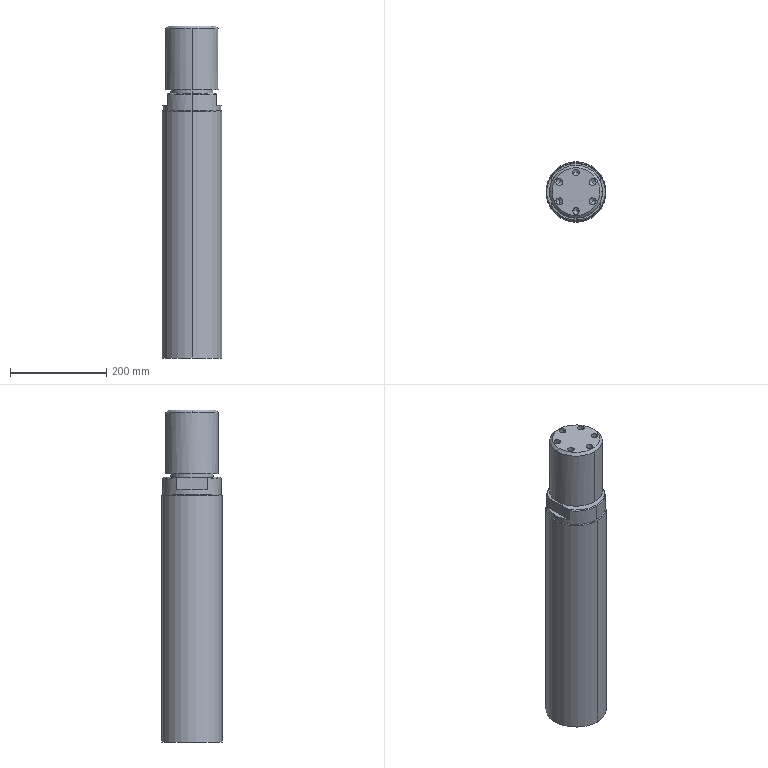Part | SolidWorks | features BaseBody 1, CirPattern 1, HoleWzd 1 | 1 solid | 46 faces | box 125 x 125 x 690 mm | volume 7968385 mm3 | cylinder 20 | cone 18 | plane 8 | commonest cylinder face diameters 14 x12 88 x2 110 x2 121.5 x2 125 x2
STEP:
#1=CARTESIAN_POINT('',(-38.141,13.938,152.));
#2=VERTEX_POINT('',#1);
#3=CARTESIAN_POINT('',(-31.141,26.062,152.));
#4=VERTEX_POINT('',#3);
#5=CARTESIAN_POINT('',(-34.641,20.,152.));
#6=DIRECTION('',(0.,0.,1.));
#7=DIRECTION('',(0.5,0.866,0.));
#8=AXIS2_PLACEMENT_3D('',#5,#6,#7);
#9=CIRCLE('',#8,7.);
#10=EDGE_CURVE('',#2,#4,#9,.T.);
#11=ORIENTED_EDGE('',*,*,#10,.F.);
#12=CARTESIAN_POINT('',(-38.141,13.938,190.));
#13=VERTEX_POINT('',#12);
#14=CARTESIAN_POINT('',(-38.141,13.938,190.));
#15=DIRECTION('',(0.,0.,1.));
#16=VECTOR('',#15,1000.);
#17=LINE('',#14,#16);
#18=EDGE_CURVE('',#2,#13,#17,.T.);
#19=ORIENTED_EDGE('',*,*,#18,.T.);
#20=CARTESIAN_POINT('',(-31.141,26.062,190.));
#21=VERTEX_POINT('',#20);
#22=CARTESIAN_POINT('',(-34.641,20.,190.));
#23=DIRECTION('',(0.,0.,1.));
#24=DIRECTION('',(0.5,0.866,0.));
#25=AXIS2_PLACEMENT_3D('',#22,#23,#24);
#26=CIRCLE('',#25,7.);
#27=EDGE_CURVE('',#13,#21,#26,.T.);
#28=ORIENTED_EDGE('',*,*,#27,.T.);
#29=CARTESIAN_POINT('',(-31.141,26.062,190.));
#30=DIRECTION('',(0.,0.,1.));
#31=VECTOR('',#30,1000.);
#32=LINE('',#29,#31);
#33=EDGE_CURVE('',#4,#21,#32,.T.);
#34=ORIENTED_EDGE('',*,*,#33,.F.);
#35=EDGE_LOOP('',(#11,#19,#28,#34));
#36=FACE_OUTER_BOUND('',#35,.T.);
#37=CARTESIAN_POINT('',(-34.641,20.,190.));
#38=DIRECTION('',(0.,0.,1.));
#39=DIRECTION('',(0.5,0.866,0.));
#40=AXIS2_PLACEMENT_3D('',#37,#38,#39);
#41=CYLINDRICAL_SURFACE('',#40,7.);
#42=ADVANCED_FACE('',(#36),#41,.F.);
#43=CARTESIAN_POINT('',(-34.641,20.,147.794));
#44=VERTEX_POINT('',#43);
#45=CARTESIAN_POINT('',(-31.141,26.062,152.));
#46=DIRECTION('',(0.4286,0.7423,0.515));
#47=VECTOR('',#46,1000.);
#48=LINE('',#45,#47);
#49=EDGE_CURVE('',#44,#4,#48,.T.);
#50=ORIENTED_EDGE('',*,*,#49,.F.);
#51=CARTESIAN_POINT('',(-38.141,13.938,152.));
#52=DIRECTION('',(-0.4286,-0.7423,0.515));
#53=VECTOR('',#52,1000.);
#54=LINE('',#51,#53);
#55=EDGE_CURVE('',#44,#2,#54,.T.);
#56=ORIENTED_EDGE('',*,*,#55,.T.);
#57=ORIENTED_EDGE('',*,*,#10,.T.);
#58=EDGE_LOOP('',(#50,#56,#57));
#59=FACE_OUTER_BOUND('',#58,.T.);
#60=CARTESIAN_POINT('',(-34.641,20.,152.));
#61=DIRECTION('',(0.,0.,1.));
#62=DIRECTION('',(0.5,0.866,0.));
#63=AXIS2_PLACEMENT_3D('',#60,#61,#62);
#64=CONICAL_SURFACE('',#63,7.,1.03);
#65=ADVANCED_FACE('',(#59),#64,.F.);
#66=CARTESIAN_POINT('',(-31.141,-26.062,152.));
#67=VERTEX_POINT('',#66);
#68=CARTESIAN_POINT('',(-38.141,-13.938,152.));
#69=VERTEX_POINT('',#68);
#70=CARTESIAN_POINT('',(-34.641,-20.,152.));
#71=DIRECTION('',(0.,0.,1.));
#72=DIRECTION('',(-0.5,0.866,0.));
#73=AXIS2_PLACEMENT_3D('',#70,#71,#72);
#74=CIRCLE('',#73,7.);
#75=EDGE_CURVE('',#67,#69,#74,.T.);
#76=ORIENTED_EDGE('',*,*,#75,.F.);
#77=CARTESIAN_POINT('',(-31.141,-26.062,190.));
#78=VERTEX_POINT('',#77);
#79=CARTESIAN_POINT('',(-31.141,-26.062,190.));
#80=DIRECTION('',(0.,0.,1.));
#81=VECTOR('',#80,1000.);
#82=LINE('',#79,#81);
#83=EDGE_CURVE('',#67,#78,#82,.T.);
#84=ORIENTED_EDGE('',*,*,#83,.T.);
#85=CARTESIAN_POINT('',(-38.141,-13.938,190.));
#86=VERTEX_POINT('',#85);
#87=CARTESIAN_POINT('',(-34.641,-20.,190.));
#88=DIRECTION('',(0.,0.,1.));
#89=DIRECTION('',(-0.5,0.866,0.));
#90=AXIS2_PLACEMENT_3D('',#87,#88,#89);
#91=CIRCLE('',#90,7.);
#92=EDGE_CURVE('',#78,#86,#91,.T.);
#93=ORIENTED_EDGE('',*,*,#92,.T.);
#94=CARTESIAN_POINT('',(-38.141,-13.938,190.));
#95=DIRECTION('',(0.,0.,1.));
#96=VECTOR('',#95,1000.);
#97=LINE('',#94,#96);
#98=EDGE_CURVE('',#69,#86,#97,.T.);
#99=ORIENTED_EDGE('',*,*,#98,.F.);
#100=EDGE_LOOP('',(#76,#84,#93,#99));
#101=FACE_OUTER_BOUND('',#100,.T.);
#102=CARTESIAN_POINT('',(-34.641,-20.,190.));
#103=DIRECTION('',(0.,0.,1.));
#104=DIRECTION('',(-0.5,0.866,0.));
#105=AXIS2_PLACEMENT_3D('',#102,#103,#104);
#106=CYLINDRICAL_SURFACE('',#105,7.);
#107=ADVANCED_FACE('',(#101),#106,.F.);
#108=CARTESIAN_POINT('',(-34.641,-20.,147.794));
#109=VERTEX_POINT('',#108);
#110=CARTESIAN_POINT('',(-38.141,-13.938,152.));
#111=DIRECTION('',(-0.4286,0.7423,0.515));
#112=VECTOR('',#111,1000.);
#113=LINE('',#110,#112);
#114=EDGE_CURVE('',#109,#69,#113,.T.);
#115=ORIENTED_EDGE('',*,*,#114,.F.);
#116=CARTESIAN_POINT('',(-31.141,-26.062,152.));
#117=DIRECTION('',(0.4286,-0.7423,0.515));
#118=VECTOR('',#117,1000.);
#119=LINE('',#116,#118);
#120=EDGE_CURVE('',#109,#67,#119,.T.);
#121=ORIENTED_EDGE('',*,*,#120,.T.);
#122=ORIENTED_EDGE('',*,*,#75,.T.);
#123=EDGE_LOOP('',(#115,#121,#122));
#124=FACE_OUTER_BOUND('',#123,.T.);
#125=CARTESIAN_POINT('',(-34.641,-20.,152.));
#126=DIRECTION('',(0.,0.,1.));
#127=DIRECTION('',(-0.5,0.866,0.));
#128=AXIS2_PLACEMENT_3D('',#125,#126,#127);
#129=CONICAL_SURFACE('',#128,7.,1.03);
#130=ADVANCED_FACE('',(#124),#129,.F.);
#131=CARTESIAN_POINT('',(7.,-40.,152.));
#132=VERTEX_POINT('',#131);
#133=CARTESIAN_POINT('',(-7.,-40.,152.));
#134=VERTEX_POINT('',#133);
#135=CARTESIAN_POINT('',(0.,-40.,152.));
#136=DIRECTION('',(0.,0.,1.));
#137=DIRECTION('',(-1.,0.,0.));
#138=AXIS2_PLACEMENT_3D('',#135,#136,#137);
#139=CIRCLE('',#138,7.);
#140=EDGE_CURVE('',#132,#134,#139,.T.);
#141=ORIENTED_EDGE('',*,*,#140,.F.);
#142=CARTESIAN_POINT('',(7.,-40.,190.));
#143=VERTEX_POINT('',#142);
#144=CARTESIAN_POINT('',(7.,-40.,190.));
#145=DIRECTION('',(0.,0.,1.));
#146=VECTOR('',#145,1000.);
#147=LINE('',#144,#146);
#148=EDGE_CURVE('',#132,#143,#147,.T.);
#149=ORIENTED_EDGE('',*,*,#148,.T.);
#150=CARTESIAN_POINT('',(-7.,-40.,190.));
#151=VERTEX_POINT('',#150);
#152=CARTESIAN_POINT('',(0.,-40.,190.));
#153=DIRECTION('',(0.,0.,1.));
#154=DIRECTION('',(-1.,0.,0.));
#155=AXIS2_PLACEMENT_3D('',#152,#153,#154);
#156=CIRCLE('',#155,7.);
#157=EDGE_CURVE('',#143,#151,#156,.T.);
#158=ORIENTED_EDGE('',*,*,#157,.T.);
#159=CARTESIAN_POINT('',(-7.,-40.,190.));
#160=DIRECTION('',(0.,0.,1.));
#161=VECTOR('',#160,1000.);
#162=LINE('',#159,#161);
#163=EDGE_CURVE('',#134,#151,#162,.T.);
#164=ORIENTED_EDGE('',*,*,#163,.F.);
#165=EDGE_LOOP('',(#141,#149,#158,#164));
#166=FACE_OUTER_BOUND('',#165,.T.);
#167=CARTESIAN_POINT('',(0.,-40.,190.));
#168=DIRECTION('',(0.,0.,1.));
#169=DIRECTION('',(-1.,0.,0.));
#170=AXIS2_PLACEMENT_3D('',#167,#168,#169);
#171=CYLINDRICAL_SURFACE('',#170,7.);
#172=ADVANCED_FACE('',(#166),#171,.F.);
#173=CARTESIAN_POINT('',(0.,-40.,147.794));
#174=VERTEX_POINT('',#173);
#175=CARTESIAN_POINT('',(-7.,-40.,152.));
#176=DIRECTION('',(-0.8572,0.,0.515));
#177=VECTOR('',#176,1000.);
#178=LINE('',#175,#177);
#179=EDGE_CURVE('',#174,#134,#178,.T.);
#180=ORIENTED_EDGE('',*,*,#179,.F.);
#181=CARTESIAN_POINT('',(7.,-40.,152.));
#182=DIRECTION('',(0.8572,0.,0.515));
#183=VECTOR('',#182,1000.);
#184=LINE('',#181,#183);
#185=EDGE_CURVE('',#174,#132,#184,.T.);
#186=ORIENTED_EDGE('',*,*,#185,.T.);
#187=ORIENTED_EDGE('',*,*,#140,.T.);
#188=EDGE_LOOP('',(#180,#186,#187));
#189=FACE_OUTER_BOUND('',#188,.T.);
#190=CARTESIAN_POINT('',(0.,-40.,152.));
#191=DIRECTION('',(0.,0.,1.));
#192=DIRECTION('',(-1.,0.,0.));
#193=AXIS2_PLACEMENT_3D('',#190,#191,#192);
#194=CONICAL_SURFACE('',#193,7.,1.03);
#195=ADVANCED_FACE('',(#189),#194,.F.);
#196=CARTESIAN_POINT('',(38.141,-13.938,152.));
#197=VERTEX_POINT('',#196);
#198=CARTESIAN_POINT('',(31.141,-26.062,152.));
#199=VERTEX_POINT('',#198);
#200=CARTESIAN_POINT('',(34.641,-20.,152.));
#201=DIRECTION('',(0.,0.,1.));
#202=DIRECTION('',(-0.5,-0.866,0.));
#203=AXIS2_PLACEMENT_3D('',#200,#201,#202);
#204=CIRCLE('',#203,7.);
#205=EDGE_CURVE('',#197,#199,#204,.T.);
#206=ORIENTED_EDGE('',*,*,#205,.F.);
#207=CARTESIAN_POINT('',(38.141,-13.938,190.));
#208=VERTEX_POINT('',#207);
#209=CARTESIAN_POINT('',(38.141,-13.938,190.));
#210=DIRECTION('',(0.,0.,1.));
#211=VECTOR('',#210,1000.);
#212=LINE('',#209,#211);
#213=EDGE_CURVE('',#197,#208,#212,.T.);
#214=ORIENTED_EDGE('',*,*,#213,.T.);
#215=CARTESIAN_POINT('',(31.141,-26.062,190.));
#216=VERTEX_POINT('',#215);
#217=CARTESIAN_POINT('',(34.641,-20.,190.));
#218=DIRECTION('',(0.,0.,1.));
#219=DIRECTION('',(-0.5,-0.866,0.));
#220=AXIS2_PLACEMENT_3D('',#217,#218,#219);
#221=CIRCLE('',#220,7.);
#222=EDGE_CURVE('',#208,#216,#221,.T.);
#223=ORIENTED_EDGE('',*,*,#222,.T.);
#224=CARTESIAN_POINT('',(31.141,-26.062,190.));
#225=DIRECTION('',(0.,0.,1.));
#226=VECTOR('',#225,1000.);
#227=LINE('',#224,#226);
#228=EDGE_CURVE('',#199,#216,#227,.T.);
#229=ORIENTED_EDGE('',*,*,#228,.F.);
#230=EDGE_LOOP('',(#206,#214,#223,#229));
#231=FACE_OUTER_BOUND('',#230,.T.);
#232=CARTESIAN_POINT('',(34.641,-20.,190.));
#233=DIRECTION('',(0.,0.,1.));
#234=DIRECTION('',(-0.5,-0.866,0.));
#235=AXIS2_PLACEMENT_3D('',#232,#233,#234);
#236=CYLINDRICAL_SURFACE('',#235,7.);
#237=ADVANCED_FACE('',(#231),#236,.F.);
#238=CARTESIAN_POINT('',(34.641,-20.,147.794));
#239=VERTEX_POINT('',#238);
#240=CARTESIAN_POINT('',(31.141,-26.062,152.));
#241=DIRECTION('',(-0.4286,-0.7423,0.515));
#242=VECTOR('',#241,1000.);
#243=LINE('',#240,#242);
#244=EDGE_CURVE('',#239,#199,#243,.T.);
#245=ORIENTED_EDGE('',*,*,#244,.F.);
#246=CARTESIAN_POINT('',(38.141,-13.938,152.));
#247=DIRECTION('',(0.4286,0.7423,0.515));
#248=VECTOR('',#247,1000.);
#249=LINE('',#246,#248);
#250=EDGE_CURVE('',#239,#197,#249,.T.);
#251=ORIENTED_EDGE('',*,*,#250,.T.);
#252=ORIENTED_EDGE('',*,*,#205,.T.);
#253=EDGE_LOOP('',(#245,#251,#252));
#254=FACE_OUTER_BOUND('',#253,.T.);
#255=CARTESIAN_POINT('',(34.641,-20.,152.));
#256=DIRECTION('',(0.,0.,1.));
#257=DIRECTION('',(-0.5,-0.866,0.));
#258=AXIS2_PLACEMENT_3D('',#255,#256,#257);
#259=CONICAL_SURFACE('',#258,7.,1.03);
#260=ADVANCED_FACE('',(#254),#259,.F.);
#261=CARTESIAN_POINT('',(31.141,26.062,152.));
#262=VERTEX_POINT('',#261);
#263=CARTESIAN_POINT('',(38.141,13.938,152.));
#264=VERTEX_POINT('',#263);
#265=CARTESIAN_POINT('',(34.641,20.,152.));
#266=DIRECTION('',(0.,0.,1.));
#267=DIRECTION('',(0.5,-0.866,0.));
#268=AXIS2_PLACEMENT_3D('',#265,#266,#267);
#269=CIRCLE('',#268,7.);
#270=EDGE_CURVE('',#262,#264,#269,.T.);
#271=ORIENTED_EDGE('',*,*,#270,.F.);
#272=CARTESIAN_POINT('',(31.141,26.062,190.));
#273=VERTEX_POINT('',#272);
#274=CARTESIAN_POINT('',(31.141,26.062,190.));
#275=DIRECTION('',(0.,0.,1.));
#276=VECTOR('',#275,1000.);
#277=LINE('',#274,#276);
#278=EDGE_CURVE('',#262,#273,#277,.T.);
#279=ORIENTED_EDGE('',*,*,#278,.T.);
#280=CARTESIAN_POINT('',(38.141,13.938,190.));
#281=VERTEX_POINT('',#280);
#282=CARTESIAN_POINT('',(34.641,20.,190.));
#283=DIRECTION('',(0.,0.,1.));
#284=DIRECTION('',(0.5,-0.866,0.));
#285=AXIS2_PLACEMENT_3D('',#282,#283,#284);
#286=CIRCLE('',#285,7.);
#287=EDGE_CURVE('',#273,#281,#286,.T.);
#288=ORIENTED_EDGE('',*,*,#287,.T.);
#289=CARTESIAN_POINT('',(38.141,13.938,190.));
#290=DIRECTION('',(0.,0.,1.));
#291=VECTOR('',#290,1000.);
#292=LINE('',#289,#291);
#293=EDGE_CURVE('',#264,#281,#292,.T.);
#294=ORIENTED_EDGE('',*,*,#293,.F.);
#295=EDGE_LOOP('',(#271,#279,#288,#294));
#296=FACE_OUTER_BOUND('',#295,.T.);
#297=CARTESIAN_POINT('',(34.641,20.,190.));
#298=DIRECTION('',(0.,0.,1.));
#299=DIRECTION('',(0.5,-0.866,0.));
#300=AXIS2_PLACEMENT_3D('',#297,#298,#299);
#301=CYLINDRICAL_SURFACE('',#300,7.);
#302=ADVANCED_FACE('',(#296),#301,.F.);
#303=CARTESIAN_POINT('',(34.641,20.,147.794));
#304=VERTEX_POINT('',#303);
#305=CARTESIAN_POINT('',(38.141,13.938,152.));
#306=DIRECTION('',(0.4286,-0.7423,0.515));
#307=VECTOR('',#306,1000.);
#308=LINE('',#305,#307);
#309=EDGE_CURVE('',#304,#264,#308,.T.);
#310=ORIENTED_EDGE('',*,*,#309,.F.);
#311=CARTESIAN_POINT('',(31.141,26.062,152.));
#312=DIRECTION('',(-0.4286,0.7423,0.515));
#313=VECTOR('',#312,1000.);
#314=LINE('',#311,#313);
#315=EDGE_CURVE('',#304,#262,#314,.T.);
#316=ORIENTED_EDGE('',*,*,#315,.T.);
#317=ORIENTED_EDGE('',*,*,#270,.T.);
#318=EDGE_LOOP('',(#310,#316,#317));
#319=FACE_OUTER_BOUND('',#318,.T.);
#320=CARTESIAN_POINT('',(34.641,20.,152.));
#321=DIRECTION('',(0.,0.,1.));
#322=DIRECTION('',(0.5,-0.866,0.));
#323=AXIS2_PLACEMENT_3D('',#320,#321,#322);
#324=CONICAL_SURFACE('',#323,7.,1.03);
#325=ADVANCED_FACE('',(#319),#324,.F.);
#326=CARTESIAN_POINT('',(-7.,40.,152.));
#327=VERTEX_POINT('',#326);
#328=CARTESIAN_POINT('',(7.,40.,152.));
#329=VERTEX_POINT('',#328);
#330=CARTESIAN_POINT('',(0.,40.,152.));
#331=DIRECTION('',(0.,0.,1.));
#332=DIRECTION('',(1.,0.,0.));
#333=AXIS2_PLACEMENT_3D('',#330,#331,#332);
#334=CIRCLE('',#333,7.);
#335=EDGE_CURVE('',#327,#329,#334,.T.);
#336=ORIENTED_EDGE('',*,*,#335,.F.);
#337=CARTESIAN_POINT('',(-7.,40.,190.));
#338=VERTEX_POINT('',#337);
#339=CARTESIAN_POINT('',(-7.,40.,190.));
#340=DIRECTION('',(0.,0.,1.));
#341=VECTOR('',#340,1000.);
#342=LINE('',#339,#341);
#343=EDGE_CURVE('',#327,#338,#342,.T.);
#344=ORIENTED_EDGE('',*,*,#343,.T.);
#345=CARTESIAN_POINT('',(7.,40.,190.));
#346=VERTEX_POINT('',#345);
#347=CARTESIAN_POINT('',(0.,40.,190.));
#348=DIRECTION('',(0.,0.,1.));
#349=DIRECTION('',(1.,0.,0.));
#350=AXIS2_PLACEMENT_3D('',#347,#348,#349);
#351=CIRCLE('',#350,7.);
#352=EDGE_CURVE('',#338,#346,#351,.T.);
#353=ORIENTED_EDGE('',*,*,#352,.T.);
#354=CARTESIAN_POINT('',(7.,40.,190.));
#355=DIRECTION('',(0.,0.,1.));
#356=VECTOR('',#355,1000.);
#357=LINE('',#354,#356);
#358=EDGE_CURVE('',#329,#346,#357,.T.);
#359=ORIENTED_EDGE('',*,*,#358,.F.);
#360=EDGE_LOOP('',(#336,#344,#353,#359));
#361=FACE_OUTER_BOUND('',#360,.T.);
#362=CARTESIAN_POINT('',(0.,40.,190.));
#363=DIRECTION('',(0.,0.,1.));
#364=DIRECTION('',(1.,0.,0.));
#365=AXIS2_PLACEMENT_3D('',#362,#363,#364);
#366=CYLINDRICAL_SURFACE('',#365,7.);
#367=ADVANCED_FACE('',(#361),#366,.F.);
#368=CARTESIAN_POINT('',(0.,40.,147.794));
#369=VERTEX_POINT('',#368);
#370=CARTESIAN_POINT('',(7.,40.,152.));
#371=DIRECTION('',(0.8572,0.,0.515));
#372=VECTOR('',#371,1000.);
#373=LINE('',#370,#372);
#374=EDGE_CURVE('',#369,#329,#373,.T.);
#375=ORIENTED_EDGE('',*,*,#374,.F.);
#376=CARTESIAN_POINT('',(-7.,40.,152.));
#377=DIRECTION('',(-0.8572,0.,0.515));
#378=VECTOR('',#377,1000.);
#379=LINE('',#376,#378);
#380=EDGE_CURVE('',#369,#327,#379,.T.);
#381=ORIENTED_EDGE('',*,*,#380,.T.);
#382=ORIENTED_EDGE('',*,*,#335,.T.);
#383=EDGE_LOOP('',(#375,#381,#382));
#384=FACE_OUTER_BOUND('',#383,.T.);
#385=CARTESIAN_POINT('',(0.,40.,152.));
#386=DIRECTION('',(0.,0.,1.));
#387=DIRECTION('',(1.,0.,0.));
#388=AXIS2_PLACEMENT_3D('',#385,#386,#387);
#389=CONICAL_SURFACE('',#388,7.,1.03);
#390=ADVANCED_FACE('',(#384),#389,.F.);
#391=CARTESIAN_POINT('',(0.,62.5,12.5));
#392=VERTEX_POINT('',#391);
#393=CARTESIAN_POINT('',(0.,-62.5,12.5));
#394=VERTEX_POINT('',#393);
#395=CARTESIAN_POINT('',(0.,0.,12.5));
#396=DIRECTION('',(0.,0.,-1.));
#397=DIRECTION('',(0.,1.,0.));
#398=AXIS2_PLACEMENT_3D('',#395,#396,#397);
#399=CIRCLE('',#398,62.5);
#400=EDGE_CURVE('',#392,#394,#399,.T.);
#401=ORIENTED_EDGE('',*,*,#400,.T.);
#402=CARTESIAN_POINT('',(0.,-62.5,-500.));
#403=VERTEX_POINT('',#402);
#404=CARTESIAN_POINT('',(0.,-62.5,-500.));
#405=DIRECTION('',(0.,0.,-1.));
#406=VECTOR('',#405,1000.);
#407=LINE('',#404,#406);
#408=EDGE_CURVE('',#394,#403,#407,.T.);
#409=ORIENTED_EDGE('',*,*,#408,.T.);
#410=CARTESIAN_POINT('',(0.,62.5,-500.));
#411=VERTEX_POINT('',#410);
#412=CARTESIAN_POINT('',(0.,0.,-500.));
#413=DIRECTION('',(0.,0.,1.));
#414=DIRECTION('',(0.,1.,0.));
#415=AXIS2_PLACEMENT_3D('',#412,#413,#414);
#416=CIRCLE('',#415,62.5);
#417=EDGE_CURVE('',#403,#411,#416,.T.);
#418=ORIENTED_EDGE('',*,*,#417,.T.);
#419=CARTESIAN_POINT('',(0.,62.5,-500.));
#420=DIRECTION('',(0.,0.,-1.));
#421=VECTOR('',#420,1000.);
#422=LINE('',#419,#421);
#423=EDGE_CURVE('',#392,#411,#422,.T.);
#424=ORIENTED_EDGE('',*,*,#423,.F.);
#425=EDGE_LOOP('',(#401,#409,#418,#424));
#426=FACE_OUTER_BOUND('',#425,.T.);
#427=CARTESIAN_POINT('',(0.,0.,-500.));
#428=DIRECTION('',(0.,0.,-1.));
#429=DIRECTION('',(0.,1.,0.));
#430=AXIS2_PLACEMENT_3D('',#427,#428,#429);
#431=CYLINDRICAL_SURFACE('',#430,62.5);
#432=ADVANCED_FACE('',(#426),#431,.T.);
#433=CARTESIAN_POINT('',(0.,60.75,14.25));
#434=VERTEX_POINT('',#433);
#435=CARTESIAN_POINT('',(0.,-60.75,14.25));
#436=VERTEX_POINT('',#435);
#437=CARTESIAN_POINT('',(0.,0.,14.25));
#438=DIRECTION('',(0.,0.,-1.));
#439=DIRECTION('',(0.,1.,0.));
#440=AXIS2_PLACEMENT_3D('',#437,#438,#439);
#441=CIRCLE('',#440,60.75);
#442=EDGE_CURVE('',#434,#436,#441,.T.);
#443=ORIENTED_EDGE('',*,*,#442,.T.);
#444=CARTESIAN_POINT('',(0.,-62.5,12.5));
#445=DIRECTION('',(0.,-0.7071,-0.7071));
#446=VECTOR('',#445,1000.);
#447=LINE('',#444,#446);
#448=EDGE_CURVE('',#436,#394,#447,.T.);
#449=ORIENTED_EDGE('',*,*,#448,.T.);
#450=ORIENTED_EDGE('',*,*,#400,.F.);
#451=CARTESIAN_POINT('',(0.,62.5,12.5));
#452=DIRECTION('',(0.,0.7071,-0.7071));
#453=VECTOR('',#452,1000.);
#454=LINE('',#451,#453);
#455=EDGE_CURVE('',#434,#392,#454,.T.);
#456=ORIENTED_EDGE('',*,*,#455,.F.);
#457=EDGE_LOOP('',(#443,#449,#450,#456));
#458=FACE_OUTER_BOUND('',#457,.T.);
#459=CARTESIAN_POINT('',(0.,0.,12.5));
#460=DIRECTION('',(0.,0.,-1.));
#461=DIRECTION('',(0.,1.,0.));
#462=AXIS2_PLACEMENT_3D('',#459,#460,#461);
#463=CONICAL_SURFACE('',#462,62.5,0.7854);
#464=ADVANCED_FACE('',(#458),#463,.T.);
#465=CARTESIAN_POINT('',(51.25,-32.619,48.25));
#466=VERTEX_POINT('',#465);
#467=CARTESIAN_POINT('',(0.,-60.75,48.25));
#468=VERTEX_POINT('',#467);
#469=CARTESIAN_POINT('',(0.,0.,48.25));
#470=DIRECTION('',(0.,0.,-1.));
#471=DIRECTION('',(0.,1.,0.));
#472=AXIS2_PLACEMENT_3D('',#469,#470,#471);
#473=CIRCLE('',#472,60.75);
#474=EDGE_CURVE('',#466,#468,#473,.T.);
#475=ORIENTED_EDGE('',*,*,#474,.T.);
#476=CARTESIAN_POINT('',(0.,-60.75,-500.));
#477=DIRECTION('',(0.,0.,-1.));
#478=VECTOR('',#477,1000.);
#479=LINE('',#476,#478);
#480=EDGE_CURVE('',#468,#436,#479,.T.);
#481=ORIENTED_EDGE('',*,*,#480,.T.);
#482=ORIENTED_EDGE('',*,*,#442,.F.);
#483=CARTESIAN_POINT('',(0.,60.75,48.25));
#484=VERTEX_POINT('',#483);
#485=CARTESIAN_POINT('',(0.,60.75,-500.));
#486=DIRECTION('',(0.,0.,-1.));
#487=VECTOR('',#486,1000.);
#488=LINE('',#485,#487);
#489=EDGE_CURVE('',#484,#434,#488,.T.);
#490=ORIENTED_EDGE('',*,*,#489,.F.);
#491=CARTESIAN_POINT('',(51.25,32.619,48.25));
#492=VERTEX_POINT('',#491);
#493=CARTESIAN_POINT('',(0.,0.,48.25));
#494=DIRECTION('',(0.,0.,-1.));
#495=DIRECTION('',(0.,1.,0.));
#496=AXIS2_PLACEMENT_3D('',#493,#494,#495);
#497=CIRCLE('',#496,60.75);
#498=EDGE_CURVE('',#484,#492,#497,.T.);
#499=ORIENTED_EDGE('',*,*,#498,.T.);
#500=CARTESIAN_POINT('',(51.25,32.619,25.));
#501=VERTEX_POINT('',#500);
#502=CARTESIAN_POINT('',(51.25,32.619,-500.));
#503=DIRECTION('',(0.,0.,-1.));
#504=VECTOR('',#503,1000.);
#505=LINE('',#502,#504);
#506=EDGE_CURVE('',#492,#501,#505,.T.);
#507=ORIENTED_EDGE('',*,*,#506,.T.);
#508=CARTESIAN_POINT('',(51.25,-32.619,25.));
#509=VERTEX_POINT('',#508);
#510=CARTESIAN_POINT('',(0.,0.,25.));
#511=DIRECTION('',(0.,0.,-1.));
#512=DIRECTION('',(0.,1.,0.));
#513=AXIS2_PLACEMENT_3D('',#510,#511,#512);
#514=CIRCLE('',#513,60.75);
#515=EDGE_CURVE('',#501,#509,#514,.T.);
#516=ORIENTED_EDGE('',*,*,#515,.T.);
#517=CARTESIAN_POINT('',(51.25,-32.619,-500.));
#518=DIRECTION('',(0.,0.,1.));
#519=VECTOR('',#518,1000.);
#520=LINE('',#517,#519);
#521=EDGE_CURVE('',#509,#466,#520,.T.);
#522=ORIENTED_EDGE('',*,*,#521,.T.);
#523=EDGE_LOOP('',(#475,#481,#482,#490,#499,#507,#516,#522));
#524=FACE_OUTER_BOUND('',#523,.T.);
#525=CARTESIAN_POINT('',(0.,0.,-500.));
#526=DIRECTION('',(0.,0.,-1.));
#527=DIRECTION('',(0.,1.,0.));
#528=AXIS2_PLACEMENT_3D('',#525,#526,#527);
#529=CYLINDRICAL_SURFACE('',#528,60.75);
#530=ADVANCED_FACE('',(#524),#529,.T.);
#531=CARTESIAN_POINT('',(0.,44.,57.));
#532=VERTEX_POINT('',#531);
#533=CARTESIAN_POINT('',(0.,-44.,57.));
#534=VERTEX_POINT('',#533);
#535=CARTESIAN_POINT('',(0.,0.,57.));
#536=DIRECTION('',(0.,0.,-1.));
#537=DIRECTION('',(0.,1.,0.));
#538=AXIS2_PLACEMENT_3D('',#535,#536,#537);
#539=CIRCLE('',#538,44.);
#540=EDGE_CURVE('',#532,#534,#539,.T.);
#541=ORIENTED_EDGE('',*,*,#540,.T.);
#542=CARTESIAN_POINT('',(0.,-44.,50.));
#543=VERTEX_POINT('',#542);
#544=CARTESIAN_POINT('',(0.,-44.,-500.));
#545=DIRECTION('',(0.,0.,-1.));
#546=VECTOR('',#545,1000.);
#547=LINE('',#544,#546);
#548=EDGE_CURVE('',#534,#543,#547,.T.);
#549=ORIENTED_EDGE('',*,*,#548,.T.);
#550=CARTESIAN_POINT('',(0.,44.,50.));
#551=VERTEX_POINT('',#550);
#552=CARTESIAN_POINT('',(0.,0.,50.));
#553=DIRECTION('',(0.,0.,-1.));
#554=DIRECTION('',(0.,1.,0.));
#555=AXIS2_PLACEMENT_3D('',#552,#553,#554);
#556=CIRCLE('',#555,44.);
#557=EDGE_CURVE('',#551,#543,#556,.T.);
#558=ORIENTED_EDGE('',*,*,#557,.F.);
#559=CARTESIAN_POINT('',(0.,44.,-500.));
#560=DIRECTION('',(0.,0.,-1.));
#561=VECTOR('',#560,1000.);
#562=LINE('',#559,#561);
#563=EDGE_CURVE('',#532,#551,#562,.T.);
#564=ORIENTED_EDGE('',*,*,#563,.F.);
#565=EDGE_LOOP('',(#541,#549,#558,#564));
#566=FACE_OUTER_BOUND('',#565,.T.);
#567=CARTESIAN_POINT('',(0.,0.,-500.));
#568=DIRECTION('',(0.,0.,-1.));
#569=DIRECTION('',(0.,1.,0.));
#570=AXIS2_PLACEMENT_3D('',#567,#568,#569);
#571=CYLINDRICAL_SURFACE('',#570,44.);
#572=ADVANCED_FACE('',(#566),#571,.T.);
#573=CARTESIAN_POINT('',(55.,0.,184.5));
#574=VERTEX_POINT('',#573);
#575=CARTESIAN_POINT('',(0.,-55.,184.5));
#576=VERTEX_POINT('',#575);
#577=CARTESIAN_POINT('',(0.,0.,184.5));
#578=DIRECTION('',(0.,0.,-1.));
#579=DIRECTION('',(0.,1.,0.));
#580=AXIS2_PLACEMENT_3D('',#577,#578,#579);
#581=CIRCLE('',#580,55.);
#582=EDGE_CURVE('',#574,#576,#581,.T.);
#583=ORIENTED_EDGE('',*,*,#582,.T.);
#584=CARTESIAN_POINT('',(0.,-55.,57.));
#585=VERTEX_POINT('',#584);
#586=CARTESIAN_POINT('',(0.,-55.,-500.));
#587=DIRECTION('',(0.,0.,-1.));
#588=VECTOR('',#587,1000.);
#589=LINE('',#586,#588);
#590=EDGE_CURVE('',#576,#585,#589,.T.);
#591=ORIENTED_EDGE('',*,*,#590,.T.);
#592=CARTESIAN_POINT('',(0.,55.,57.));
#593=VERTEX_POINT('',#592);
#594=CARTESIAN_POINT('',(0.,0.,57.));
#595=DIRECTION('',(0.,0.,-1.));
#596=DIRECTION('',(0.,1.,0.));
#597=AXIS2_PLACEMENT_3D('',#594,#595,#596);
#598=CIRCLE('',#597,55.);
#599=EDGE_CURVE('',#593,#585,#598,.T.);
#600=ORIENTED_EDGE('',*,*,#599,.F.);
#601=CARTESIAN_POINT('',(0.,55.,184.5));
#602=VERTEX_POINT('',#601);
#603=CARTESIAN_POINT('',(0.,55.,-500.));
#604=DIRECTION('',(0.,0.,-1.));
#605=VECTOR('',#604,1000.);
#606=LINE('',#603,#605);
#607=EDGE_CURVE('',#602,#593,#606,.T.);
#608=ORIENTED_EDGE('',*,*,#607,.F.);
#609=CARTESIAN_POINT('',(0.,0.,184.5));
#610=DIRECTION('',(0.,0.,-1.));
#611=DIRECTION('',(0.,1.,0.));
#612=AXIS2_PLACEMENT_3D('',#609,#610,#611);
#613=CIRCLE('',#612,55.);
#614=EDGE_CURVE('',#602,#574,#613,.T.);
#615=ORIENTED_EDGE('',*,*,#614,.T.);
#616=EDGE_LOOP('',(#583,#591,#600,#608,#615));
#617=FACE_OUTER_BOUND('',#616,.T.);
#618=CARTESIAN_POINT('',(0.,0.,-500.));
#619=DIRECTION('',(0.,0.,-1.));
#620=DIRECTION('',(0.,1.,0.));
#621=AXIS2_PLACEMENT_3D('',#618,#619,#620);
#622=CYLINDRICAL_SURFACE('',#621,55.);
#623=ADVANCED_FACE('',(#617),#622,.T.);
#624=CARTESIAN_POINT('',(-49.5,0.,190.));
#625=VERTEX_POINT('',#624);
#626=CARTESIAN_POINT('',(49.5,0.,190.));
#627=VERTEX_POINT('',#626);
#628=CARTESIAN_POINT('',(0.,0.,190.));
#629=DIRECTION('',(0.,0.,-1.));
#630=DIRECTION('',(-1.,0.,0.));
#631=AXIS2_PLACEMENT_3D('',#628,#629,#630);
#632=CIRCLE('',#631,49.5);
#633=EDGE_CURVE('',#625,#627,#632,.T.);
#634=ORIENTED_EDGE('',*,*,#633,.T.);
#635=CARTESIAN_POINT('',(55.,0.,184.5));
#636=DIRECTION('',(0.7071,0.,-0.7071));
#637=VECTOR('',#636,1000.);
#638=LINE('',#635,#637);
#639=EDGE_CURVE('',#627,#574,#638,.T.);
#640=ORIENTED_EDGE('',*,*,#639,.T.);
#641=ORIENTED_EDGE('',*,*,#614,.F.);
#642=CARTESIAN_POINT('',(-55.,0.,184.5));
#643=VERTEX_POINT('',#642);
#644=CARTESIAN_POINT('',(0.,0.,184.5));
#645=DIRECTION('',(0.,0.,-1.));
#646=DIRECTION('',(0.,1.,0.));
#647=AXIS2_PLACEMENT_3D('',#644,#645,#646);
#648=CIRCLE('',#647,55.);
#649=EDGE_CURVE('',#643,#602,#648,.T.);
#650=ORIENTED_EDGE('',*,*,#649,.F.);
#651=CARTESIAN_POINT('',(-55.,0.,184.5));
#652=DIRECTION('',(-0.7071,0.,-0.7071));
#653=VECTOR('',#652,1000.);
#654=LINE('',#651,#653);
#655=EDGE_CURVE('',#625,#643,#654,.T.);
#656=ORIENTED_EDGE('',*,*,#655,.F.);
#657=EDGE_LOOP('',(#634,#640,#641,#650,#656));
#658=FACE_OUTER_BOUND('',#657,.T.);
#659=CARTESIAN_POINT('',(0.,0.,184.5));
#660=DIRECTION('',(0.,0.,-1.));
#661=DIRECTION('',(-1.,0.,0.));
#662=AXIS2_PLACEMENT_3D('',#659,#660,#661);
#663=CONICAL_SURFACE('',#662,55.,0.7854);
#664=ADVANCED_FACE('',(#658),#663,.T.);
#665=ORIENTED_EDGE('',*,*,#408,.F.);
#666=CARTESIAN_POINT('',(0.,0.,12.5));
#667=DIRECTION('',(0.,0.,-1.));
#668=DIRECTION('',(0.,1.,0.));
#669=AXIS2_PLACEMENT_3D('',#666,#667,#668);
#670=CIRCLE('',#669,62.5);
#671=EDGE_CURVE('',#394,#392,#670,.T.);
#672=ORIENTED_EDGE('',*,*,#671,.T.);
#673=ORIENTED_EDGE('',*,*,#423,.T.);
#674=CARTESIAN_POINT('',(0.,0.,-500.));
#675=DIRECTION('',(0.,0.,1.));
#676=DIRECTION('',(0.,1.,0.));
#677=AXIS2_PLACEMENT_3D('',#674,#675,#676);
#678=CIRCLE('',#677,62.5);
#679=EDGE_CURVE('',#411,#403,#678,.T.);
#680=ORIENTED_EDGE('',*,*,#679,.T.);
#681=EDGE_LOOP('',(#665,#672,#673,#680));
#682=FACE_OUTER_BOUND('',#681,.T.);
#683=CARTESIAN_POINT('',(0.,0.,-500.));
#684=DIRECTION('',(0.,0.,-1.));
#685=DIRECTION('',(0.,1.,0.));
#686=AXIS2_PLACEMENT_3D('',#683,#684,#685);
#687=CYLINDRICAL_SURFACE('',#686,62.5);
#688=ADVANCED_FACE('',(#682),#687,.T.);
#689=ORIENTED_EDGE('',*,*,#679,.F.);
#690=ORIENTED_EDGE('',*,*,#417,.F.);
#691=EDGE_LOOP('',(#689,#690));
#692=FACE_OUTER_BOUND('',#691,.T.);
#693=CARTESIAN_POINT('',(0.,-62.5,-500.));
#694=DIRECTION('',(0.,0.,-1.));
#695=DIRECTION('',(0.,1.,0.));
#696=AXIS2_PLACEMENT_3D('',#693,#694,#695);
#697=PLANE('',#696);
#698=ADVANCED_FACE('',(#692),#697,.T.);
#699=ORIENTED_EDGE('',*,*,#448,.F.);
#700=CARTESIAN_POINT('',(0.,0.,14.25));
#701=DIRECTION('',(0.,0.,-1.));
#702=DIRECTION('',(0.,1.,0.));
#703=AXIS2_PLACEMENT_3D('',#700,#701,#702);
#704=CIRCLE('',#703,60.75);
#705=EDGE_CURVE('',#436,#434,#704,.T.);
#706=ORIENTED_EDGE('',*,*,#705,.T.);
#707=ORIENTED_EDGE('',*,*,#455,.T.);
#708=ORIENTED_EDGE('',*,*,#671,.F.);
#709=EDGE_LOOP('',(#699,#706,#707,#708));
#710=FACE_OUTER_BOUND('',#709,.T.);
#711=CARTESIAN_POINT('',(0.,0.,12.5));
#712=DIRECTION('',(0.,0.,-1.));
#713=DIRECTION('',(0.,1.,0.));
#714=AXIS2_PLACEMENT_3D('',#711,#712,#713);
#715=CONICAL_SURFACE('',#714,62.5,0.7854);
#716=ADVANCED_FACE('',(#710),#715,.T.);
#717=ORIENTED_EDGE('',*,*,#480,.F.);
#718=CARTESIAN_POINT('',(-51.25,-32.619,48.25));
#719=VERTEX_POINT('',#718);
#720=CARTESIAN_POINT('',(0.,0.,48.25));
#721=DIRECTION('',(0.,0.,-1.));
#722=DIRECTION('',(0.,1.,0.));
#723=AXIS2_PLACEMENT_3D('',#720,#721,#722);
#724=CIRCLE('',#723,60.75);
#725=EDGE_CURVE('',#468,#719,#724,.T.);
#726=ORIENTED_EDGE('',*,*,#725,.T.);
#727=CARTESIAN_POINT('',(-51.25,-32.619,25.));
#728=VERTEX_POINT('',#727);
#729=CARTESIAN_POINT('',(-51.25,-32.619,-500.));
#730=DIRECTION('',(0.,0.,-1.));
#731=VECTOR('',#730,1000.);
#732=LINE('',#729,#731);
#733=EDGE_CURVE('',#719,#728,#732,.T.);
#734=ORIENTED_EDGE('',*,*,#733,.T.);
#735=CARTESIAN_POINT('',(-51.25,32.619,25.));
#736=VERTEX_POINT('',#735);
#737=CARTESIAN_POINT('',(0.,0.,25.));
#738=DIRECTION('',(0.,0.,-1.));
#739=DIRECTION('',(0.,1.,0.));
#740=AXIS2_PLACEMENT_3D('',#737,#738,#739);
#741=CIRCLE('',#740,60.75);
#742=EDGE_CURVE('',#728,#736,#741,.T.);
#743=ORIENTED_EDGE('',*,*,#742,.T.);
#744=CARTESIAN_POINT('',(-51.25,32.619,48.25));
#745=VERTEX_POINT('',#744);
#746=CARTESIAN_POINT('',(-51.25,32.619,-500.));
#747=DIRECTION('',(0.,0.,1.));
#748=VECTOR('',#747,1000.);
#749=LINE('',#746,#748);
#750=EDGE_CURVE('',#736,#745,#749,.T.);
#751=ORIENTED_EDGE('',*,*,#750,.T.);
#752=CARTESIAN_POINT('',(0.,0.,48.25));
#753=DIRECTION('',(0.,0.,-1.));
#754=DIRECTION('',(0.,1.,0.));
#755=AXIS2_PLACEMENT_3D('',#752,#753,#754);
#756=CIRCLE('',#755,60.75);
#757=EDGE_CURVE('',#745,#484,#756,.T.);
#758=ORIENTED_EDGE('',*,*,#757,.T.);
#759=ORIENTED_EDGE('',*,*,#489,.T.);
#760=ORIENTED_EDGE('',*,*,#705,.F.);
#761=EDGE_LOOP('',(#717,#726,#734,#743,#751,#758,#759,#760));
#762=FACE_OUTER_BOUND('',#761,.T.);
#763=CARTESIAN_POINT('',(0.,0.,-500.));
#764=DIRECTION('',(0.,0.,-1.));
#765=DIRECTION('',(0.,1.,0.));
#766=AXIS2_PLACEMENT_3D('',#763,#764,#765);
#767=CYLINDRICAL_SURFACE('',#766,60.75);
#768=ADVANCED_FACE('',(#762),#767,.T.);
#769=CARTESIAN_POINT('',(51.25,-29.231,50.));
#770=VERTEX_POINT('',#769);
#771=CARTESIAN_POINT('',(51.25,29.231,50.));
#772=VERTEX_POINT('',#771);
#773=CARTESIAN_POINT('',(51.25,32.619,50.));
#774=DIRECTION('',(0.,1.,0.));
#775=VECTOR('',#774,1000.);
#776=LINE('',#773,#775);
#777=EDGE_CURVE('',#770,#772,#776,.T.);
#778=ORIENTED_EDGE('',*,*,#777,.F.);
#779=CARTESIAN_POINT('',(51.25,-32.619,48.25));
#780=CARTESIAN_POINT('',(51.25,-31.479,48.862));
#781=CARTESIAN_POINT('',(51.25,-30.35,49.445));
#782=CARTESIAN_POINT('',(51.25,-29.231,50.));
#783=B_SPLINE_CURVE_WITH_KNOTS('',3,(#779,#780,#781,#782),.UNSPECIFIED.,.F.,.F.,(4,4),(0.,1.),.UNSPECIFIED.);
#784=EDGE_CURVE('',#466,#770,#783,.T.);
#785=ORIENTED_EDGE('',*,*,#784,.F.);
#786=ORIENTED_EDGE('',*,*,#521,.F.);
#787=CARTESIAN_POINT('',(51.25,32.619,25.));
#788=DIRECTION('',(0.,-1.,0.));
#789=VECTOR('',#788,1000.);
#790=LINE('',#787,#789);
#791=EDGE_CURVE('',#501,#509,#790,.T.);
#792=ORIENTED_EDGE('',*,*,#791,.F.);
#793=ORIENTED_EDGE('',*,*,#506,.F.);
#794=CARTESIAN_POINT('',(51.25,29.231,50.));
#795=CARTESIAN_POINT('',(51.25,30.35,49.445));
#796=CARTESIAN_POINT('',(51.25,31.479,48.862));
#797=CARTESIAN_POINT('',(51.25,32.619,48.25));
#798=B_SPLINE_CURVE_WITH_KNOTS('',3,(#794,#795,#796,#797),.UNSPECIFIED.,.F.,.F.,(4,4),(0.,1.),.UNSPECIFIED.);
#799=EDGE_CURVE('',#772,#492,#798,.T.);
#800=ORIENTED_EDGE('',*,*,#799,.F.);
#801=EDGE_LOOP('',(#778,#785,#786,#792,#793,#800));
#802=FACE_OUTER_BOUND('',#801,.T.);
#803=CARTESIAN_POINT('',(51.25,32.619,25.));
#804=DIRECTION('',(-1.,0.,0.));
#805=DIRECTION('',(0.,0.,1.));
#806=AXIS2_PLACEMENT_3D('',#803,#804,#805);
#807=PLANE('',#806);
#808=ADVANCED_FACE('',(#802),#807,.F.);
#809=ORIENTED_EDGE('',*,*,#515,.F.);
#810=ORIENTED_EDGE('',*,*,#791,.T.);
#811=EDGE_LOOP('',(#809,#810));
#812=FACE_OUTER_BOUND('',#811,.T.);
#813=CARTESIAN_POINT('',(0.,0.,25.));
#814=DIRECTION('',(0.,0.,1.));
#815=DIRECTION('',(1.,0.,0.));
#816=AXIS2_PLACEMENT_3D('',#813,#814,#815);
#817=PLANE('',#816);
#818=ADVANCED_FACE('',(#812),#817,.T.);
#819=ORIENTED_EDGE('',*,*,#799,.T.);
#820=ORIENTED_EDGE('',*,*,#498,.F.);
#821=ORIENTED_EDGE('',*,*,#757,.F.);
#822=CARTESIAN_POINT('',(-51.25,29.231,50.));
#823=VERTEX_POINT('',#822);
#824=CARTESIAN_POINT('',(-51.25,32.619,48.25));
#825=CARTESIAN_POINT('',(-51.25,31.479,48.862));
#826=CARTESIAN_POINT('',(-51.25,30.35,49.445));
#827=CARTESIAN_POINT('',(-51.25,29.231,50.));
#828=B_SPLINE_CURVE_WITH_KNOTS('',3,(#824,#825,#826,#827),.UNSPECIFIED.,.F.,.F.,(4,4),(0.,1.),.UNSPECIFIED.);
#829=EDGE_CURVE('',#745,#823,#828,.T.);
#830=ORIENTED_EDGE('',*,*,#829,.T.);
#831=CARTESIAN_POINT('',(0.,0.,50.));
#832=DIRECTION('',(0.,0.,-1.));
#833=DIRECTION('',(-1.,0.,0.));
#834=AXIS2_PLACEMENT_3D('',#831,#832,#833);
#835=CIRCLE('',#834,59.);
#836=EDGE_CURVE('',#823,#772,#835,.T.);
#837=ORIENTED_EDGE('',*,*,#836,.T.);
#838=EDGE_LOOP('',(#819,#820,#821,#830,#837));
#839=FACE_OUTER_BOUND('',#838,.T.);
#840=CARTESIAN_POINT('',(0.,0.,48.25));
#841=DIRECTION('',(0.,0.,-1.));
#842=DIRECTION('',(-1.,0.,0.));
#843=AXIS2_PLACEMENT_3D('',#840,#841,#842);
#844=CONICAL_SURFACE('',#843,60.75,0.7854);
#845=ADVANCED_FACE('',(#839),#844,.T.);
#846=CARTESIAN_POINT('',(-51.25,-29.231,50.));
#847=VERTEX_POINT('',#846);
#848=CARTESIAN_POINT('',(-51.25,-29.231,50.));
#849=CARTESIAN_POINT('',(-51.25,-30.35,49.445));
#850=CARTESIAN_POINT('',(-51.25,-31.479,48.862));
#851=CARTESIAN_POINT('',(-51.25,-32.619,48.25));
#852=B_SPLINE_CURVE_WITH_KNOTS('',3,(#848,#849,#850,#851),.UNSPECIFIED.,.F.,.F.,(4,4),(0.,1.),.UNSPECIFIED.);
#853=EDGE_CURVE('',#847,#719,#852,.T.);
#854=ORIENTED_EDGE('',*,*,#853,.T.);
#855=ORIENTED_EDGE('',*,*,#725,.F.);
#856=ORIENTED_EDGE('',*,*,#474,.F.);
#857=ORIENTED_EDGE('',*,*,#784,.T.);
#858=CARTESIAN_POINT('',(0.,0.,50.));
#859=DIRECTION('',(0.,0.,-1.));
#860=DIRECTION('',(-1.,0.,0.));
#861=AXIS2_PLACEMENT_3D('',#858,#859,#860);
#862=CIRCLE('',#861,59.);
#863=EDGE_CURVE('',#770,#847,#862,.T.);
#864=ORIENTED_EDGE('',*,*,#863,.T.);
#865=EDGE_LOOP('',(#854,#855,#856,#857,#864));
#866=FACE_OUTER_BOUND('',#865,.T.);
#867=CARTESIAN_POINT('',(0.,0.,48.25));
#868=DIRECTION('',(0.,0.,-1.));
#869=DIRECTION('',(-1.,0.,0.));
#870=AXIS2_PLACEMENT_3D('',#867,#868,#869);
#871=CONICAL_SURFACE('',#870,60.75,0.7854);
#872=ADVANCED_FACE('',(#866),#871,.T.);
#873=CARTESIAN_POINT('',(-51.25,32.619,50.));
#874=DIRECTION('',(0.,-1.,0.));
#875=VECTOR('',#874,1000.);
#876=LINE('',#873,#875);
#877=EDGE_CURVE('',#823,#847,#876,.T.);
#878=ORIENTED_EDGE('',*,*,#877,.F.);
#879=ORIENTED_EDGE('',*,*,#829,.F.);
#880=ORIENTED_EDGE('',*,*,#750,.F.);
#881=CARTESIAN_POINT('',(-51.25,32.619,25.));
#882=DIRECTION('',(0.,1.,0.));
#883=VECTOR('',#882,1000.);
#884=LINE('',#881,#883);
#885=EDGE_CURVE('',#728,#736,#884,.T.);
#886=ORIENTED_EDGE('',*,*,#885,.F.);
#887=ORIENTED_EDGE('',*,*,#733,.F.);
#888=ORIENTED_EDGE('',*,*,#853,.F.);
#889=EDGE_LOOP('',(#878,#879,#880,#886,#887,#888));
#890=FACE_OUTER_BOUND('',#889,.T.);
#891=CARTESIAN_POINT('',(-51.25,32.619,25.));
#892=DIRECTION('',(1.,0.,0.));
#893=DIRECTION('',(0.,0.,-1.));
#894=AXIS2_PLACEMENT_3D('',#891,#892,#893);
#895=PLANE('',#894);
#896=ADVANCED_FACE('',(#890),#895,.F.);
#897=ORIENTED_EDGE('',*,*,#742,.F.);
#898=ORIENTED_EDGE('',*,*,#885,.T.);
#899=EDGE_LOOP('',(#897,#898));
#900=FACE_OUTER_BOUND('',#899,.T.);
#901=CARTESIAN_POINT('',(0.,0.,25.));
#902=DIRECTION('',(0.,0.,1.));
#903=DIRECTION('',(1.,0.,0.));
#904=AXIS2_PLACEMENT_3D('',#901,#902,#903);
#905=PLANE('',#904);
#906=ADVANCED_FACE('',(#900),#905,.T.);
#907=ORIENTED_EDGE('',*,*,#557,.T.);
#908=CARTESIAN_POINT('',(0.,0.,50.));
#909=DIRECTION('',(0.,0.,-1.));
#910=DIRECTION('',(0.,1.,0.));
#911=AXIS2_PLACEMENT_3D('',#908,#909,#910);
#912=CIRCLE('',#911,44.);
#913=EDGE_CURVE('',#543,#551,#912,.T.);
#914=ORIENTED_EDGE('',*,*,#913,.T.);
#915=EDGE_LOOP('',(#907,#914));
#916=FACE_BOUND('',#915,.T.);
#917=ORIENTED_EDGE('',*,*,#877,.T.);
#918=ORIENTED_EDGE('',*,*,#863,.F.);
#919=ORIENTED_EDGE('',*,*,#777,.T.);
#920=ORIENTED_EDGE('',*,*,#836,.F.);
#921=EDGE_LOOP('',(#917,#918,#919,#920));
#922=FACE_OUTER_BOUND('',#921,.T.);
#923=CARTESIAN_POINT('',(0.,-44.,50.));
#924=DIRECTION('',(0.,0.,1.));
#925=DIRECTION('',(0.,-1.,0.));
#926=AXIS2_PLACEMENT_3D('',#923,#924,#925);
#927=PLANE('',#926);
#928=ADVANCED_FACE('',(#916,#922),#927,.T.);
#929=ORIENTED_EDGE('',*,*,#548,.F.);
#930=CARTESIAN_POINT('',(0.,0.,57.));
#931=DIRECTION('',(0.,0.,-1.));
#932=DIRECTION('',(0.,1.,0.));
#933=AXIS2_PLACEMENT_3D('',#930,#931,#932);
#934=CIRCLE('',#933,44.);
#935=EDGE_CURVE('',#534,#532,#934,.T.);
#936=ORIENTED_EDGE('',*,*,#935,.T.);
#937=ORIENTED_EDGE('',*,*,#563,.T.);
#938=ORIENTED_EDGE('',*,*,#913,.F.);
#939=EDGE_LOOP('',(#929,#936,#937,#938));
#940=FACE_OUTER_BOUND('',#939,.T.);
#941=CARTESIAN_POINT('',(0.,0.,-500.));
#942=DIRECTION('',(0.,0.,-1.));
#943=DIRECTION('',(0.,1.,0.));
#944=AXIS2_PLACEMENT_3D('',#941,#942,#943);
#945=CYLINDRICAL_SURFACE('',#944,44.);
#946=ADVANCED_FACE('',(#940),#945,.T.);
#947=ORIENTED_EDGE('',*,*,#540,.F.);
#948=ORIENTED_EDGE('',*,*,#935,.F.);
#949=EDGE_LOOP('',(#947,#948));
#950=FACE_BOUND('',#949,.T.);
#951=ORIENTED_EDGE('',*,*,#599,.T.);
#952=CARTESIAN_POINT('',(0.,0.,57.));
#953=DIRECTION('',(0.,0.,-1.));
#954=DIRECTION('',(0.,1.,0.));
#955=AXIS2_PLACEMENT_3D('',#952,#953,#954);
#956=CIRCLE('',#955,55.);
#957=EDGE_CURVE('',#585,#593,#956,.T.);
#958=ORIENTED_EDGE('',*,*,#957,.T.);
#959=EDGE_LOOP('',(#951,#958));
#960=FACE_OUTER_BOUND('',#959,.T.);
#961=CARTESIAN_POINT('',(0.,-55.,57.));
#962=DIRECTION('',(0.,0.,-1.));
#963=DIRECTION('',(0.,1.,0.));
#964=AXIS2_PLACEMENT_3D('',#961,#962,#963);
#965=PLANE('',#964);
#966=ADVANCED_FACE('',(#950,#960),#965,.T.);
#967=ORIENTED_EDGE('',*,*,#590,.F.);
#968=CARTESIAN_POINT('',(0.,0.,184.5));
#969=DIRECTION('',(0.,0.,-1.));
#970=DIRECTION('',(0.,1.,0.));
#971=AXIS2_PLACEMENT_3D('',#968,#969,#970);
#972=CIRCLE('',#971,55.);
#973=EDGE_CURVE('',#576,#643,#972,.T.);
#974=ORIENTED_EDGE('',*,*,#973,.T.);
#975=ORIENTED_EDGE('',*,*,#649,.T.);
#976=ORIENTED_EDGE('',*,*,#607,.T.);
#977=ORIENTED_EDGE('',*,*,#957,.F.);
#978=EDGE_LOOP('',(#967,#974,#975,#976,#977));
#979=FACE_OUTER_BOUND('',#978,.T.);
#980=CARTESIAN_POINT('',(0.,0.,-500.));
#981=DIRECTION('',(0.,0.,-1.));
#982=DIRECTION('',(0.,1.,0.));
#983=AXIS2_PLACEMENT_3D('',#980,#981,#982);
#984=CYLINDRICAL_SURFACE('',#983,55.);
#985=ADVANCED_FACE('',(#979),#984,.T.);
#986=ORIENTED_EDGE('',*,*,#639,.F.);
#987=CARTESIAN_POINT('',(0.,0.,190.));
#988=DIRECTION('',(0.,0.,-1.));
#989=DIRECTION('',(-1.,0.,0.));
#990=AXIS2_PLACEMENT_3D('',#987,#988,#989);
#991=CIRCLE('',#990,49.5);
#992=EDGE_CURVE('',#627,#625,#991,.T.);
#993=ORIENTED_EDGE('',*,*,#992,.T.);
#994=ORIENTED_EDGE('',*,*,#655,.T.);
#995=ORIENTED_EDGE('',*,*,#973,.F.);
#996=ORIENTED_EDGE('',*,*,#582,.F.);
#997=EDGE_LOOP('',(#986,#993,#994,#995,#996));
#998=FACE_OUTER_BOUND('',#997,.T.);
#999=CARTESIAN_POINT('',(0.,0.,184.5));
#1000=DIRECTION('',(0.,0.,-1.));
#1001=DIRECTION('',(-1.,0.,0.));
#1002=AXIS2_PLACEMENT_3D('',#999,#1000,#1001);
#1003=CONICAL_SURFACE('',#1002,55.,0.7854);
#1004=ADVANCED_FACE('',(#998),#1003,.T.);
#1005=CARTESIAN_POINT('',(-34.641,20.,190.));
#1006=DIRECTION('',(0.,0.,1.));
#1007=DIRECTION('',(0.5,0.866,0.));
#1008=AXIS2_PLACEMENT_3D('',#1005,#1006,#1007);
#1009=CIRCLE('',#1008,7.);
#1010=EDGE_CURVE('',#21,#13,#1009,.T.);
#1011=ORIENTED_EDGE('',*,*,#1010,.F.);
#1012=ORIENTED_EDGE('',*,*,#27,.F.);
#1013=EDGE_LOOP('',(#1011,#1012));
#1014=FACE_BOUND('',#1013,.T.);
#1015=CARTESIAN_POINT('',(-34.641,-20.,190.));
#1016=DIRECTION('',(0.,0.,1.));
#1017=DIRECTION('',(-0.5,0.866,0.));
#1018=AXIS2_PLACEMENT_3D('',#1015,#1016,#1017);
#1019=CIRCLE('',#1018,7.);
#1020=EDGE_CURVE('',#86,#78,#1019,.T.);
#1021=ORIENTED_EDGE('',*,*,#1020,.F.);
#1022=ORIENTED_EDGE('',*,*,#92,.F.);
#1023=EDGE_LOOP('',(#1021,#1022));
#1024=FACE_BOUND('',#1023,.T.);
#1025=CARTESIAN_POINT('',(0.,-40.,190.));
#1026=DIRECTION('',(0.,0.,1.));
#1027=DIRECTION('',(-1.,0.,0.));
#1028=AXIS2_PLACEMENT_3D('',#1025,#1026,#1027);
#1029=CIRCLE('',#1028,7.);
#1030=EDGE_CURVE('',#151,#143,#1029,.T.);
#1031=ORIENTED_EDGE('',*,*,#1030,.F.);
#1032=ORIENTED_EDGE('',*,*,#157,.F.);
#1033=EDGE_LOOP('',(#1031,#1032));
#1034=FACE_BOUND('',#1033,.T.);
#1035=CARTESIAN_POINT('',(34.641,-20.,190.));
#1036=DIRECTION('',(0.,0.,1.));
#1037=DIRECTION('',(-0.5,-0.866,0.));
#1038=AXIS2_PLACEMENT_3D('',#1035,#1036,#1037);
#1039=CIRCLE('',#1038,7.);
#1040=EDGE_CURVE('',#216,#208,#1039,.T.);
#1041=ORIENTED_EDGE('',*,*,#1040,.F.);
#1042=ORIENTED_EDGE('',*,*,#222,.F.);
#1043=EDGE_LOOP('',(#1041,#1042));
#1044=FACE_BOUND('',#1043,.T.);
#1045=CARTESIAN_POINT('',(34.641,20.,190.));
#1046=DIRECTION('',(0.,0.,1.));
#1047=DIRECTION('',(0.5,-0.866,0.));
#1048=AXIS2_PLACEMENT_3D('',#1045,#1046,#1047);
#1049=CIRCLE('',#1048,7.);
#1050=EDGE_CURVE('',#281,#273,#1049,.T.);
#1051=ORIENTED_EDGE('',*,*,#1050,.F.);
#1052=ORIENTED_EDGE('',*,*,#287,.F.);
#1053=EDGE_LOOP('',(#1051,#1052));
#1054=FACE_BOUND('',#1053,.T.);
#1055=CARTESIAN_POINT('',(0.,40.,190.));
#1056=DIRECTION('',(0.,0.,1.));
#1057=DIRECTION('',(1.,0.,0.));
#1058=AXIS2_PLACEMENT_3D('',#1055,#1056,#1057);
#1059=CIRCLE('',#1058,7.);
#1060=EDGE_CURVE('',#346,#338,#1059,.T.);
#1061=ORIENTED_EDGE('',*,*,#1060,.F.);
#1062=ORIENTED_EDGE('',*,*,#352,.F.);
#1063=EDGE_LOOP('',(#1061,#1062));
#1064=FACE_BOUND('',#1063,.T.);
#1065=ORIENTED_EDGE('',*,*,#633,.F.);
#1066=ORIENTED_EDGE('',*,*,#992,.F.);
#1067=EDGE_LOOP('',(#1065,#1066));
#1068=FACE_OUTER_BOUND('',#1067,.T.);
#1069=CARTESIAN_POINT('',(0.,0.,190.));
#1070=DIRECTION('',(0.,0.,1.));
#1071=DIRECTION('',(0.,-1.,0.));
#1072=AXIS2_PLACEMENT_3D('',#1069,#1070,#1071);
#1073=PLANE('',#1072);
#1074=ADVANCED_FACE('',(#1014,#1024,#1034,#1044,#1054,#1064,#1068),#1073,.T.);
#1075=ORIENTED_EDGE('',*,*,#380,.F.);
#1076=ORIENTED_EDGE('',*,*,#374,.T.);
#1077=CARTESIAN_POINT('',(0.,40.,152.));
#1078=DIRECTION('',(0.,0.,1.));
#1079=DIRECTION('',(1.,0.,0.));
#1080=AXIS2_PLACEMENT_3D('',#1077,#1078,#1079);
#1081=CIRCLE('',#1080,7.);
#1082=EDGE_CURVE('',#329,#327,#1081,.T.);
#1083=ORIENTED_EDGE('',*,*,#1082,.T.);
#1084=EDGE_LOOP('',(#1075,#1076,#1083));
#1085=FACE_OUTER_BOUND('',#1084,.T.);
#1086=CARTESIAN_POINT('',(0.,40.,152.));
#1087=DIRECTION('',(0.,0.,1.));
#1088=DIRECTION('',(1.,0.,0.));
#1089=AXIS2_PLACEMENT_3D('',#1086,#1087,#1088);
#1090=CONICAL_SURFACE('',#1089,7.,1.03);
#1091=ADVANCED_FACE('',(#1085),#1090,.F.);
#1092=ORIENTED_EDGE('',*,*,#343,.F.);
#1093=ORIENTED_EDGE('',*,*,#1082,.F.);
#1094=ORIENTED_EDGE('',*,*,#358,.T.);
#1095=ORIENTED_EDGE('',*,*,#1060,.T.);
#1096=EDGE_LOOP('',(#1092,#1093,#1094,#1095));
#1097=FACE_OUTER_BOUND('',#1096,.T.);
#1098=CARTESIAN_POINT('',(0.,40.,190.));
#1099=DIRECTION('',(0.,0.,1.));
#1100=DIRECTION('',(1.,0.,0.));
#1101=AXIS2_PLACEMENT_3D('',#1098,#1099,#1100);
#1102=CYLINDRICAL_SURFACE('',#1101,7.);
#1103=ADVANCED_FACE('',(#1097),#1102,.F.);
#1104=ORIENTED_EDGE('',*,*,#315,.F.);
#1105=ORIENTED_EDGE('',*,*,#309,.T.);
#1106=CARTESIAN_POINT('',(34.641,20.,152.));
#1107=DIRECTION('',(0.,0.,1.));
#1108=DIRECTION('',(0.5,-0.866,0.));
#1109=AXIS2_PLACEMENT_3D('',#1106,#1107,#1108);
#1110=CIRCLE('',#1109,7.);
#1111=EDGE_CURVE('',#264,#262,#1110,.T.);
#1112=ORIENTED_EDGE('',*,*,#1111,.T.);
#1113=EDGE_LOOP('',(#1104,#1105,#1112));
#1114=FACE_OUTER_BOUND('',#1113,.T.);
#1115=CARTESIAN_POINT('',(34.641,20.,152.));
#1116=DIRECTION('',(0.,0.,1.));
#1117=DIRECTION('',(0.5,-0.866,0.));
#1118=AXIS2_PLACEMENT_3D('',#1115,#1116,#1117);
#1119=CONICAL_SURFACE('',#1118,7.,1.03);
#1120=ADVANCED_FACE('',(#1114),#1119,.F.);
#1121=ORIENTED_EDGE('',*,*,#278,.F.);
#1122=ORIENTED_EDGE('',*,*,#1111,.F.);
#1123=ORIENTED_EDGE('',*,*,#293,.T.);
#1124=ORIENTED_EDGE('',*,*,#1050,.T.);
#1125=EDGE_LOOP('',(#1121,#1122,#1123,#1124));
#1126=FACE_OUTER_BOUND('',#1125,.T.);
#1127=CARTESIAN_POINT('',(34.641,20.,190.));
#1128=DIRECTION('',(0.,0.,1.));
#1129=DIRECTION('',(0.5,-0.866,0.));
#1130=AXIS2_PLACEMENT_3D('',#1127,#1128,#1129);
#1131=CYLINDRICAL_SURFACE('',#1130,7.);
#1132=ADVANCED_FACE('',(#1126),#1131,.F.);
#1133=ORIENTED_EDGE('',*,*,#250,.F.);
#1134=ORIENTED_EDGE('',*,*,#244,.T.);
#1135=CARTESIAN_POINT('',(34.641,-20.,152.));
#1136=DIRECTION('',(0.,0.,1.));
#1137=DIRECTION('',(-0.5,-0.866,0.));
#1138=AXIS2_PLACEMENT_3D('',#1135,#1136,#1137);
#1139=CIRCLE('',#1138,7.);
#1140=EDGE_CURVE('',#199,#197,#1139,.T.);
#1141=ORIENTED_EDGE('',*,*,#1140,.T.);
#1142=EDGE_LOOP('',(#1133,#1134,#1141));
#1143=FACE_OUTER_BOUND('',#1142,.T.);
#1144=CARTESIAN_POINT('',(34.641,-20.,152.));
#1145=DIRECTION('',(0.,0.,1.));
#1146=DIRECTION('',(-0.5,-0.866,0.));
#1147=AXIS2_PLACEMENT_3D('',#1144,#1145,#1146);
#1148=CONICAL_SURFACE('',#1147,7.,1.03);
#1149=ADVANCED_FACE('',(#1143),#1148,.F.);
#1150=ORIENTED_EDGE('',*,*,#213,.F.);
#1151=ORIENTED_EDGE('',*,*,#1140,.F.);
#1152=ORIENTED_EDGE('',*,*,#228,.T.);
#1153=ORIENTED_EDGE('',*,*,#1040,.T.);
#1154=EDGE_LOOP('',(#1150,#1151,#1152,#1153));
#1155=FACE_OUTER_BOUND('',#1154,.T.);
#1156=CARTESIAN_POINT('',(34.641,-20.,190.));
#1157=DIRECTION('',(0.,0.,1.));
#1158=DIRECTION('',(-0.5,-0.866,0.));
#1159=AXIS2_PLACEMENT_3D('',#1156,#1157,#1158);
#1160=CYLINDRICAL_SURFACE('',#1159,7.);
#1161=ADVANCED_FACE('',(#1155),#1160,.F.);
#1162=ORIENTED_EDGE('',*,*,#185,.F.);
#1163=ORIENTED_EDGE('',*,*,#179,.T.);
#1164=CARTESIAN_POINT('',(0.,-40.,152.));
#1165=DIRECTION('',(0.,0.,1.));
#1166=DIRECTION('',(-1.,0.,0.));
#1167=AXIS2_PLACEMENT_3D('',#1164,#1165,#1166);
#1168=CIRCLE('',#1167,7.);
#1169=EDGE_CURVE('',#134,#132,#1168,.T.);
#1170=ORIENTED_EDGE('',*,*,#1169,.T.);
#1171=EDGE_LOOP('',(#1162,#1163,#1170));
#1172=FACE_OUTER_BOUND('',#1171,.T.);
#1173=CARTESIAN_POINT('',(0.,-40.,152.));
#1174=DIRECTION('',(0.,0.,1.));
#1175=DIRECTION('',(-1.,0.,0.));
#1176=AXIS2_PLACEMENT_3D('',#1173,#1174,#1175);
#1177=CONICAL_SURFACE('',#1176,7.,1.03);
#1178=ADVANCED_FACE('',(#1172),#1177,.F.);
#1179=ORIENTED_EDGE('',*,*,#148,.F.);
#1180=ORIENTED_EDGE('',*,*,#1169,.F.);
#1181=ORIENTED_EDGE('',*,*,#163,.T.);
#1182=ORIENTED_EDGE('',*,*,#1030,.T.);
#1183=EDGE_LOOP('',(#1179,#1180,#1181,#1182));
#1184=FACE_OUTER_BOUND('',#1183,.T.);
#1185=CARTESIAN_POINT('',(0.,-40.,190.));
#1186=DIRECTION('',(0.,0.,1.));
#1187=DIRECTION('',(-1.,0.,0.));
#1188=AXIS2_PLACEMENT_3D('',#1185,#1186,#1187);
#1189=CYLINDRICAL_SURFACE('',#1188,7.);
#1190=ADVANCED_FACE('',(#1184),#1189,.F.);
#1191=ORIENTED_EDGE('',*,*,#120,.F.);
#1192=ORIENTED_EDGE('',*,*,#114,.T.);
#1193=CARTESIAN_POINT('',(-34.641,-20.,152.));
#1194=DIRECTION('',(0.,0.,1.));
#1195=DIRECTION('',(-0.5,0.866,0.));
#1196=AXIS2_PLACEMENT_3D('',#1193,#1194,#1195);
#1197=CIRCLE('',#1196,7.);
#1198=EDGE_CURVE('',#69,#67,#1197,.T.);
#1199=ORIENTED_EDGE('',*,*,#1198,.T.);
#1200=EDGE_LOOP('',(#1191,#1192,#1199));
#1201=FACE_OUTER_BOUND('',#1200,.T.);
#1202=CARTESIAN_POINT('',(-34.641,-20.,152.));
#1203=DIRECTION('',(0.,0.,1.));
#1204=DIRECTION('',(-0.5,0.866,0.));
#1205=AXIS2_PLACEMENT_3D('',#1202,#1203,#1204);
#1206=CONICAL_SURFACE('',#1205,7.,1.03);
#1207=ADVANCED_FACE('',(#1201),#1206,.F.);
#1208=ORIENTED_EDGE('',*,*,#83,.F.);
#1209=ORIENTED_EDGE('',*,*,#1198,.F.);
#1210=ORIENTED_EDGE('',*,*,#98,.T.);
#1211=ORIENTED_EDGE('',*,*,#1020,.T.);
#1212=EDGE_LOOP('',(#1208,#1209,#1210,#1211));
#1213=FACE_OUTER_BOUND('',#1212,.T.);
#1214=CARTESIAN_POINT('',(-34.641,-20.,190.));
#1215=DIRECTION('',(0.,0.,1.));
#1216=DIRECTION('',(-0.5,0.866,0.));
#1217=AXIS2_PLACEMENT_3D('',#1214,#1215,#1216);
#1218=CYLINDRICAL_SURFACE('',#1217,7.);
#1219=ADVANCED_FACE('',(#1213),#1218,.F.);
#1220=ORIENTED_EDGE('',*,*,#55,.F.);
#1221=ORIENTED_EDGE('',*,*,#49,.T.);
#1222=CARTESIAN_POINT('',(-34.641,20.,152.));
#1223=DIRECTION('',(0.,0.,1.));
#1224=DIRECTION('',(0.5,0.866,0.));
#1225=AXIS2_PLACEMENT_3D('',#1222,#1223,#1224);
#1226=CIRCLE('',#1225,7.);
#1227=EDGE_CURVE('',#4,#2,#1226,.T.);
#1228=ORIENTED_EDGE('',*,*,#1227,.T.);
#1229=EDGE_LOOP('',(#1220,#1221,#1228));
#1230=FACE_OUTER_BOUND('',#1229,.T.);
#1231=CARTESIAN_POINT('',(-34.641,20.,152.));
#1232=DIRECTION('',(0.,0.,1.));
#1233=DIRECTION('',(0.5,0.866,0.));
#1234=AXIS2_PLACEMENT_3D('',#1231,#1232,#1233);
#1235=CONICAL_SURFACE('',#1234,7.,1.03);
#1236=ADVANCED_FACE('',(#1230),#1235,.F.);
#1237=ORIENTED_EDGE('',*,*,#18,.F.);
#1238=ORIENTED_EDGE('',*,*,#1227,.F.);
#1239=ORIENTED_EDGE('',*,*,#33,.T.);
#1240=ORIENTED_EDGE('',*,*,#1010,.T.);
#1241=EDGE_LOOP('',(#1237,#1238,#1239,#1240));
#1242=FACE_OUTER_BOUND('',#1241,.T.);
#1243=CARTESIAN_POINT('',(-34.641,20.,190.));
#1244=DIRECTION('',(0.,0.,1.));
#1245=DIRECTION('',(0.5,0.866,0.));
#1246=AXIS2_PLACEMENT_3D('',#1243,#1244,#1245);
#1247=CYLINDRICAL_SURFACE('',#1246,7.);
#1248=ADVANCED_FACE('',(#1242),#1247,.F.);
#1249=CLOSED_SHELL('',(#42,#65,#107,#130,#172,#195,#237,#260,#302,#325,#367,#390,#432,#464,#530,#572,#623,#664,#688,#698,#716,#768,#808,#818,#845,#872,#896,#906,#928,#946,#966,#985,#1004,#1074,#1091,#1103,#1120,#1132,#1149,#1161,#1178,#1190,#1207,#1219,#1236,#1248));
#1250=MANIFOLD_SOLID_BREP('',#1249);
#1251=CARTESIAN_POINT('',(0.,0.,0.));
#1252=DIRECTION('',(0.,0.,1.));
#1253=DIRECTION('',(1.,0.,0.));
#1254=AXIS2_PLACEMENT_3D('',#1251,#1252,#1253);
#1255=(LENGTH_UNIT()NAMED_UNIT(*)SI_UNIT(.MILLI.,.METRE.));
#1256=UNCERTAINTY_MEASURE_WITH_UNIT(LENGTH_MEASURE(0.00001),#1255,'','');
#1257=(NAMED_UNIT(*)PLANE_ANGLE_UNIT()SI_UNIT($,.RADIAN.));
#1258=(NAMED_UNIT(*)SI_UNIT($,.STERADIAN.)SOLID_ANGLE_UNIT());
#1259=(GEOMETRIC_REPRESENTATION_CONTEXT(3)GLOBAL_UNCERTAINTY_ASSIGNED_CONTEXT((#1256))GLOBAL_UNIT_ASSIGNED_CONTEXT((#1255,#1257,#1258))REPRESENTATION_CONTEXT('',''));
#1260=ADVANCED_BREP_SHAPE_REPRESENTATION('',(#1250,#1254),#1259);